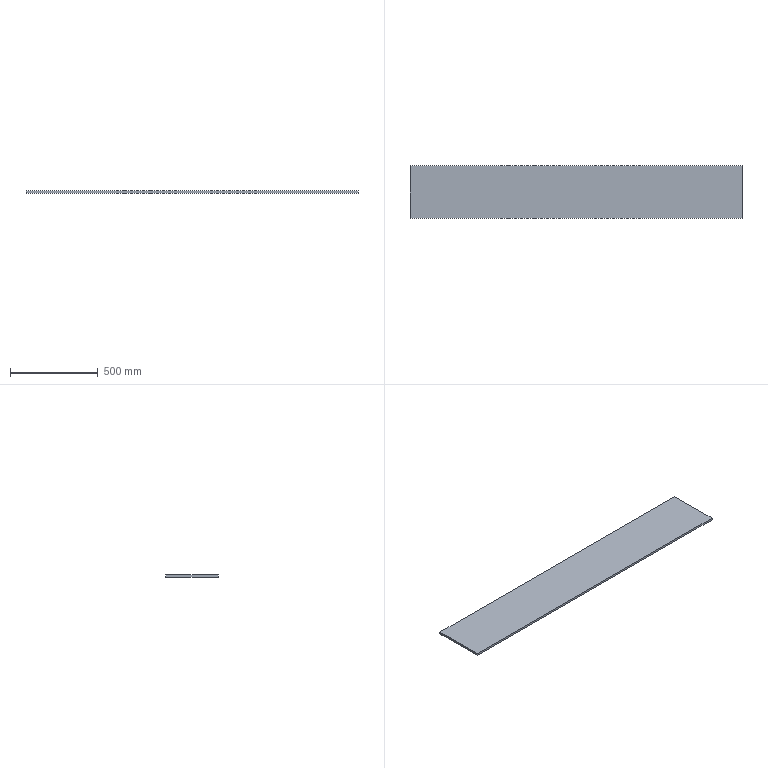Part | STEP file | 04-Steel plate | 1 solid | 6 faces | box 1888 x 300 x 12 mm | volume 6796800 mm3 | plane 6
STEP:
#1=CARTESIAN_POINT('',(0.,0.,0.));
#2=DIRECTION('',(0.,0.,1.));
#3=DIRECTION('',(1.,0.,0.));
#4=AXIS2_PLACEMENT_3D('',#1,#2,#3);
#5=CARTESIAN_POINT('',(0.,0.,0.));
#6=VERTEX_POINT('',#5);
#7=CARTESIAN_POINT('',(0.,-300.,0.));
#8=VERTEX_POINT('',#7);
#9=CARTESIAN_POINT('',(0.,0.,0.));
#10=DIRECTION('',(0.,-1.,0.));
#11=VECTOR('',#10,1.);
#12=LINE('',#9,#11);
#13=CARTESIAN_POINT('',(0.,0.,12.));
#14=DIRECTION('',(1.,0.,0.));
#15=DIRECTION('',(0.,1.,0.));
#16=AXIS2_PLACEMENT_3D('',#13,#14,#15);
#17=PLANE('',#16);
#18=CARTESIAN_POINT('',(0.,-12.));
#19=DIRECTION('',(-1.,0.));
#20=VECTOR('',#19,1.);
#21=LINE('',#18,#20);
#22=(GEOMETRIC_REPRESENTATION_CONTEXT(2)PARAMETRIC_REPRESENTATION_CONTEXT()REPRESENTATION_CONTEXT('',''));
#23=DEFINITIONAL_REPRESENTATION('',(#21),#22);
#24=PCURVE('',#17,#23);
#25=CARTESIAN_POINT('',(0.,0.,0.));
#26=DIRECTION('',(0.,0.,1.));
#27=DIRECTION('',(1.,0.,0.));
#28=AXIS2_PLACEMENT_3D('',#25,#26,#27);
#29=PLANE('',#28);
#30=CARTESIAN_POINT('',(0.,0.));
#31=DIRECTION('',(0.,-1.));
#32=VECTOR('',#31,1.);
#33=LINE('',#30,#32);
#34=(GEOMETRIC_REPRESENTATION_CONTEXT(2)PARAMETRIC_REPRESENTATION_CONTEXT()REPRESENTATION_CONTEXT('',''));
#35=DEFINITIONAL_REPRESENTATION('',(#33),#34);
#36=PCURVE('',#29,#35);
#37=SURFACE_CURVE('',#12,(#24,#36),.PCURVE_S1.);
#38=EDGE_CURVE('',#6,#8,#37,.T.);
#39=ORIENTED_EDGE('',*,*,#38,.T.);
#40=CARTESIAN_POINT('',(0.,-300.,12.));
#41=VERTEX_POINT('',#40);
#42=CARTESIAN_POINT('',(0.,-300.,12.));
#43=DIRECTION('',(0.,0.,-1.));
#44=VECTOR('',#43,1.);
#45=LINE('',#42,#44);
#46=CARTESIAN_POINT('',(-300.,0.));
#47=DIRECTION('',(0.,-1.));
#48=VECTOR('',#47,1.);
#49=LINE('',#46,#48);
#50=(GEOMETRIC_REPRESENTATION_CONTEXT(2)PARAMETRIC_REPRESENTATION_CONTEXT()REPRESENTATION_CONTEXT('',''));
#51=DEFINITIONAL_REPRESENTATION('',(#49),#50);
#52=PCURVE('',#17,#51);
#53=CARTESIAN_POINT('',(0.,-300.,12.));
#54=DIRECTION('',(0.,1.,0.));
#55=DIRECTION('',(0.,0.,1.));
#56=AXIS2_PLACEMENT_3D('',#53,#54,#55);
#57=PLANE('',#56);
#58=CARTESIAN_POINT('',(0.,0.));
#59=DIRECTION('',(-1.,0.));
#60=VECTOR('',#59,1.);
#61=LINE('',#58,#60);
#62=(GEOMETRIC_REPRESENTATION_CONTEXT(2)PARAMETRIC_REPRESENTATION_CONTEXT()REPRESENTATION_CONTEXT('',''));
#63=DEFINITIONAL_REPRESENTATION('',(#61),#62);
#64=PCURVE('',#57,#63);
#65=SURFACE_CURVE('',#45,(#52,#64),.PCURVE_S1.);
#66=EDGE_CURVE('',#41,#8,#65,.T.);
#67=ORIENTED_EDGE('',*,*,#66,.F.);
#68=CARTESIAN_POINT('',(0.,0.,12.));
#69=VERTEX_POINT('',#68);
#70=CARTESIAN_POINT('',(0.,0.,12.));
#71=DIRECTION('',(0.,-1.,0.));
#72=VECTOR('',#71,1.);
#73=LINE('',#70,#72);
#74=CARTESIAN_POINT('',(0.,0.));
#75=DIRECTION('',(-1.,0.));
#76=VECTOR('',#75,1.);
#77=LINE('',#74,#76);
#78=(GEOMETRIC_REPRESENTATION_CONTEXT(2)PARAMETRIC_REPRESENTATION_CONTEXT()REPRESENTATION_CONTEXT('',''));
#79=DEFINITIONAL_REPRESENTATION('',(#77),#78);
#80=PCURVE('',#17,#79);
#81=CARTESIAN_POINT('',(0.,0.,12.));
#82=DIRECTION('',(0.,0.,1.));
#83=DIRECTION('',(1.,0.,0.));
#84=AXIS2_PLACEMENT_3D('',#81,#82,#83);
#85=PLANE('',#84);
#86=CARTESIAN_POINT('',(0.,0.));
#87=DIRECTION('',(0.,-1.));
#88=VECTOR('',#87,1.);
#89=LINE('',#86,#88);
#90=(GEOMETRIC_REPRESENTATION_CONTEXT(2)PARAMETRIC_REPRESENTATION_CONTEXT()REPRESENTATION_CONTEXT('',''));
#91=DEFINITIONAL_REPRESENTATION('',(#89),#90);
#92=PCURVE('',#85,#91);
#93=SURFACE_CURVE('',#73,(#80,#92),.PCURVE_S1.);
#94=EDGE_CURVE('',#69,#41,#93,.T.);
#95=ORIENTED_EDGE('',*,*,#94,.F.);
#96=CARTESIAN_POINT('',(0.,0.,12.));
#97=DIRECTION('',(0.,0.,-1.));
#98=VECTOR('',#97,1.);
#99=LINE('',#96,#98);
#100=CARTESIAN_POINT('',(0.,0.));
#101=DIRECTION('',(0.,-1.));
#102=VECTOR('',#101,1.);
#103=LINE('',#100,#102);
#104=(GEOMETRIC_REPRESENTATION_CONTEXT(2)PARAMETRIC_REPRESENTATION_CONTEXT()REPRESENTATION_CONTEXT('',''));
#105=DEFINITIONAL_REPRESENTATION('',(#103),#104);
#106=PCURVE('',#17,#105);
#107=CARTESIAN_POINT('',(0.,0.,12.));
#108=DIRECTION('',(0.,-1.,0.));
#109=DIRECTION('',(0.,0.,-1.));
#110=AXIS2_PLACEMENT_3D('',#107,#108,#109);
#111=PLANE('',#110);
#112=CARTESIAN_POINT('',(0.,0.));
#113=DIRECTION('',(1.,0.));
#114=VECTOR('',#113,1.);
#115=LINE('',#112,#114);
#116=(GEOMETRIC_REPRESENTATION_CONTEXT(2)PARAMETRIC_REPRESENTATION_CONTEXT()REPRESENTATION_CONTEXT('',''));
#117=DEFINITIONAL_REPRESENTATION('',(#115),#116);
#118=PCURVE('',#111,#117);
#119=SURFACE_CURVE('',#99,(#106,#118),.PCURVE_S1.);
#120=EDGE_CURVE('',#69,#6,#119,.T.);
#121=ORIENTED_EDGE('',*,*,#120,.T.);
#122=EDGE_LOOP('',(#39,#67,#95,#121));
#123=FACE_BOUND('',#122,.T.);
#124=ADVANCED_FACE('',(#123),#17,.F.);
#125=CARTESIAN_POINT('',(1888.,-300.,0.));
#126=VERTEX_POINT('',#125);
#127=CARTESIAN_POINT('',(0.,-300.,0.));
#128=DIRECTION('',(1.,0.,0.));
#129=VECTOR('',#128,1.);
#130=LINE('',#127,#129);
#131=CARTESIAN_POINT('',(-12.,0.));
#132=DIRECTION('',(0.,1.));
#133=VECTOR('',#132,1.);
#134=LINE('',#131,#133);
#135=(GEOMETRIC_REPRESENTATION_CONTEXT(2)PARAMETRIC_REPRESENTATION_CONTEXT()REPRESENTATION_CONTEXT('',''));
#136=DEFINITIONAL_REPRESENTATION('',(#134),#135);
#137=PCURVE('',#57,#136);
#138=CARTESIAN_POINT('',(0.,-300.));
#139=DIRECTION('',(1.,0.));
#140=VECTOR('',#139,1.);
#141=LINE('',#138,#140);
#142=(GEOMETRIC_REPRESENTATION_CONTEXT(2)PARAMETRIC_REPRESENTATION_CONTEXT()REPRESENTATION_CONTEXT('',''));
#143=DEFINITIONAL_REPRESENTATION('',(#141),#142);
#144=PCURVE('',#29,#143);
#145=SURFACE_CURVE('',#130,(#137,#144),.PCURVE_S1.);
#146=EDGE_CURVE('',#8,#126,#145,.T.);
#147=ORIENTED_EDGE('',*,*,#146,.T.);
#148=CARTESIAN_POINT('',(1888.,-300.,12.));
#149=VERTEX_POINT('',#148);
#150=CARTESIAN_POINT('',(1888.,-300.,12.));
#151=DIRECTION('',(0.,0.,-1.));
#152=VECTOR('',#151,1.);
#153=LINE('',#150,#152);
#154=CARTESIAN_POINT('',(0.,1888.));
#155=DIRECTION('',(-1.,0.));
#156=VECTOR('',#155,1.);
#157=LINE('',#154,#156);
#158=(GEOMETRIC_REPRESENTATION_CONTEXT(2)PARAMETRIC_REPRESENTATION_CONTEXT()REPRESENTATION_CONTEXT('',''));
#159=DEFINITIONAL_REPRESENTATION('',(#157),#158);
#160=PCURVE('',#57,#159);
#161=CARTESIAN_POINT('',(1888.,0.,12.));
#162=DIRECTION('',(-1.,0.,0.));
#163=DIRECTION('',(0.,0.,1.));
#164=AXIS2_PLACEMENT_3D('',#161,#162,#163);
#165=PLANE('',#164);
#166=CARTESIAN_POINT('',(0.,-300.));
#167=DIRECTION('',(-1.,0.));
#168=VECTOR('',#167,1.);
#169=LINE('',#166,#168);
#170=(GEOMETRIC_REPRESENTATION_CONTEXT(2)PARAMETRIC_REPRESENTATION_CONTEXT()REPRESENTATION_CONTEXT('',''));
#171=DEFINITIONAL_REPRESENTATION('',(#169),#170);
#172=PCURVE('',#165,#171);
#173=SURFACE_CURVE('',#153,(#160,#172),.PCURVE_S1.);
#174=EDGE_CURVE('',#149,#126,#173,.T.);
#175=ORIENTED_EDGE('',*,*,#174,.F.);
#176=CARTESIAN_POINT('',(0.,-300.,12.));
#177=DIRECTION('',(1.,0.,0.));
#178=VECTOR('',#177,1.);
#179=LINE('',#176,#178);
#180=CARTESIAN_POINT('',(0.,0.));
#181=DIRECTION('',(0.,1.));
#182=VECTOR('',#181,1.);
#183=LINE('',#180,#182);
#184=(GEOMETRIC_REPRESENTATION_CONTEXT(2)PARAMETRIC_REPRESENTATION_CONTEXT()REPRESENTATION_CONTEXT('',''));
#185=DEFINITIONAL_REPRESENTATION('',(#183),#184);
#186=PCURVE('',#57,#185);
#187=CARTESIAN_POINT('',(0.,-300.));
#188=DIRECTION('',(1.,0.));
#189=VECTOR('',#188,1.);
#190=LINE('',#187,#189);
#191=(GEOMETRIC_REPRESENTATION_CONTEXT(2)PARAMETRIC_REPRESENTATION_CONTEXT()REPRESENTATION_CONTEXT('',''));
#192=DEFINITIONAL_REPRESENTATION('',(#190),#191);
#193=PCURVE('',#85,#192);
#194=SURFACE_CURVE('',#179,(#186,#193),.PCURVE_S1.);
#195=EDGE_CURVE('',#41,#149,#194,.T.);
#196=ORIENTED_EDGE('',*,*,#195,.F.);
#197=ORIENTED_EDGE('',*,*,#66,.T.);
#198=EDGE_LOOP('',(#147,#175,#196,#197));
#199=FACE_BOUND('',#198,.T.);
#200=ADVANCED_FACE('',(#199),#57,.F.);
#201=CARTESIAN_POINT('',(1888.,0.,0.));
#202=VERTEX_POINT('',#201);
#203=CARTESIAN_POINT('',(1888.,0.,0.));
#204=DIRECTION('',(0.,1.,0.));
#205=VECTOR('',#204,1.);
#206=LINE('',#203,#205);
#207=CARTESIAN_POINT('',(-12.,0.));
#208=DIRECTION('',(0.,1.));
#209=VECTOR('',#208,1.);
#210=LINE('',#207,#209);
#211=(GEOMETRIC_REPRESENTATION_CONTEXT(2)PARAMETRIC_REPRESENTATION_CONTEXT()REPRESENTATION_CONTEXT('',''));
#212=DEFINITIONAL_REPRESENTATION('',(#210),#211);
#213=PCURVE('',#165,#212);
#214=CARTESIAN_POINT('',(1888.,0.));
#215=DIRECTION('',(0.,1.));
#216=VECTOR('',#215,1.);
#217=LINE('',#214,#216);
#218=(GEOMETRIC_REPRESENTATION_CONTEXT(2)PARAMETRIC_REPRESENTATION_CONTEXT()REPRESENTATION_CONTEXT('',''));
#219=DEFINITIONAL_REPRESENTATION('',(#217),#218);
#220=PCURVE('',#29,#219);
#221=SURFACE_CURVE('',#206,(#213,#220),.PCURVE_S1.);
#222=EDGE_CURVE('',#126,#202,#221,.T.);
#223=ORIENTED_EDGE('',*,*,#222,.T.);
#224=CARTESIAN_POINT('',(1888.,0.,12.));
#225=VERTEX_POINT('',#224);
#226=CARTESIAN_POINT('',(1888.,0.,12.));
#227=DIRECTION('',(0.,0.,-1.));
#228=VECTOR('',#227,1.);
#229=LINE('',#226,#228);
#230=CARTESIAN_POINT('',(0.,0.));
#231=DIRECTION('',(-1.,0.));
#232=VECTOR('',#231,1.);
#233=LINE('',#230,#232);
#234=(GEOMETRIC_REPRESENTATION_CONTEXT(2)PARAMETRIC_REPRESENTATION_CONTEXT()REPRESENTATION_CONTEXT('',''));
#235=DEFINITIONAL_REPRESENTATION('',(#233),#234);
#236=PCURVE('',#165,#235);
#237=CARTESIAN_POINT('',(0.,1888.));
#238=DIRECTION('',(1.,0.));
#239=VECTOR('',#238,1.);
#240=LINE('',#237,#239);
#241=(GEOMETRIC_REPRESENTATION_CONTEXT(2)PARAMETRIC_REPRESENTATION_CONTEXT()REPRESENTATION_CONTEXT('',''));
#242=DEFINITIONAL_REPRESENTATION('',(#240),#241);
#243=PCURVE('',#111,#242);
#244=SURFACE_CURVE('',#229,(#236,#243),.PCURVE_S1.);
#245=EDGE_CURVE('',#225,#202,#244,.T.);
#246=ORIENTED_EDGE('',*,*,#245,.F.);
#247=CARTESIAN_POINT('',(1888.,0.,12.));
#248=DIRECTION('',(0.,1.,0.));
#249=VECTOR('',#248,1.);
#250=LINE('',#247,#249);
#251=CARTESIAN_POINT('',(0.,0.));
#252=DIRECTION('',(0.,1.));
#253=VECTOR('',#252,1.);
#254=LINE('',#251,#253);
#255=(GEOMETRIC_REPRESENTATION_CONTEXT(2)PARAMETRIC_REPRESENTATION_CONTEXT()REPRESENTATION_CONTEXT('',''));
#256=DEFINITIONAL_REPRESENTATION('',(#254),#255);
#257=PCURVE('',#165,#256);
#258=CARTESIAN_POINT('',(1888.,0.));
#259=DIRECTION('',(0.,1.));
#260=VECTOR('',#259,1.);
#261=LINE('',#258,#260);
#262=(GEOMETRIC_REPRESENTATION_CONTEXT(2)PARAMETRIC_REPRESENTATION_CONTEXT()REPRESENTATION_CONTEXT('',''));
#263=DEFINITIONAL_REPRESENTATION('',(#261),#262);
#264=PCURVE('',#85,#263);
#265=SURFACE_CURVE('',#250,(#257,#264),.PCURVE_S1.);
#266=EDGE_CURVE('',#149,#225,#265,.T.);
#267=ORIENTED_EDGE('',*,*,#266,.F.);
#268=ORIENTED_EDGE('',*,*,#174,.T.);
#269=EDGE_LOOP('',(#223,#246,#267,#268));
#270=FACE_BOUND('',#269,.T.);
#271=ADVANCED_FACE('',(#270),#165,.F.);
#272=CARTESIAN_POINT('',(0.,0.,0.));
#273=DIRECTION('',(-1.,0.,0.));
#274=VECTOR('',#273,1.);
#275=LINE('',#272,#274);
#276=CARTESIAN_POINT('',(12.,0.));
#277=DIRECTION('',(0.,-1.));
#278=VECTOR('',#277,1.);
#279=LINE('',#276,#278);
#280=(GEOMETRIC_REPRESENTATION_CONTEXT(2)PARAMETRIC_REPRESENTATION_CONTEXT()REPRESENTATION_CONTEXT('',''));
#281=DEFINITIONAL_REPRESENTATION('',(#279),#280);
#282=PCURVE('',#111,#281);
#283=CARTESIAN_POINT('',(0.,0.));
#284=DIRECTION('',(-1.,0.));
#285=VECTOR('',#284,1.);
#286=LINE('',#283,#285);
#287=(GEOMETRIC_REPRESENTATION_CONTEXT(2)PARAMETRIC_REPRESENTATION_CONTEXT()REPRESENTATION_CONTEXT('',''));
#288=DEFINITIONAL_REPRESENTATION('',(#286),#287);
#289=PCURVE('',#29,#288);
#290=SURFACE_CURVE('',#275,(#282,#289),.PCURVE_S1.);
#291=EDGE_CURVE('',#202,#6,#290,.T.);
#292=ORIENTED_EDGE('',*,*,#291,.T.);
#293=ORIENTED_EDGE('',*,*,#120,.F.);
#294=CARTESIAN_POINT('',(0.,0.,12.));
#295=DIRECTION('',(-1.,0.,0.));
#296=VECTOR('',#295,1.);
#297=LINE('',#294,#296);
#298=CARTESIAN_POINT('',(0.,0.));
#299=DIRECTION('',(0.,-1.));
#300=VECTOR('',#299,1.);
#301=LINE('',#298,#300);
#302=(GEOMETRIC_REPRESENTATION_CONTEXT(2)PARAMETRIC_REPRESENTATION_CONTEXT()REPRESENTATION_CONTEXT('',''));
#303=DEFINITIONAL_REPRESENTATION('',(#301),#302);
#304=PCURVE('',#111,#303);
#305=CARTESIAN_POINT('',(0.,0.));
#306=DIRECTION('',(-1.,0.));
#307=VECTOR('',#306,1.);
#308=LINE('',#305,#307);
#309=(GEOMETRIC_REPRESENTATION_CONTEXT(2)PARAMETRIC_REPRESENTATION_CONTEXT()REPRESENTATION_CONTEXT('',''));
#310=DEFINITIONAL_REPRESENTATION('',(#308),#309);
#311=PCURVE('',#85,#310);
#312=SURFACE_CURVE('',#297,(#304,#311),.PCURVE_S1.);
#313=EDGE_CURVE('',#225,#69,#312,.T.);
#314=ORIENTED_EDGE('',*,*,#313,.F.);
#315=ORIENTED_EDGE('',*,*,#245,.T.);
#316=EDGE_LOOP('',(#292,#293,#314,#315));
#317=FACE_BOUND('',#316,.T.);
#318=ADVANCED_FACE('',(#317),#111,.F.);
#319=ORIENTED_EDGE('',*,*,#94,.T.);
#320=ORIENTED_EDGE('',*,*,#195,.T.);
#321=ORIENTED_EDGE('',*,*,#266,.T.);
#322=ORIENTED_EDGE('',*,*,#313,.T.);
#323=EDGE_LOOP('',(#319,#320,#321,#322));
#324=FACE_BOUND('',#323,.T.);
#325=ADVANCED_FACE('',(#324),#85,.T.);
#326=ORIENTED_EDGE('',*,*,#38,.F.);
#327=ORIENTED_EDGE('',*,*,#291,.F.);
#328=ORIENTED_EDGE('',*,*,#222,.F.);
#329=ORIENTED_EDGE('',*,*,#146,.F.);
#330=EDGE_LOOP('',(#326,#327,#328,#329));
#331=FACE_BOUND('',#330,.T.);
#332=ADVANCED_FACE('',(#331),#29,.F.);
#333=CLOSED_SHELL('',(#124,#200,#271,#318,#325,#332));
#334=MANIFOLD_SOLID_BREP('',#333);
#335=(LENGTH_UNIT()NAMED_UNIT(*)SI_UNIT(.MILLI.,.METRE.));
#336=UNCERTAINTY_MEASURE_WITH_UNIT(LENGTH_MEASURE(0.0000001),#335,'','');
#337=(NAMED_UNIT(*)PLANE_ANGLE_UNIT()SI_UNIT($,.RADIAN.));
#338=(NAMED_UNIT(*)SI_UNIT($,.STERADIAN.)SOLID_ANGLE_UNIT());
#339=(GEOMETRIC_REPRESENTATION_CONTEXT(3)GLOBAL_UNCERTAINTY_ASSIGNED_CONTEXT((#336))GLOBAL_UNIT_ASSIGNED_CONTEXT((#335,#337,#338))REPRESENTATION_CONTEXT('',''));
#340=ADVANCED_BREP_SHAPE_REPRESENTATION('',(#4,#334),#339);